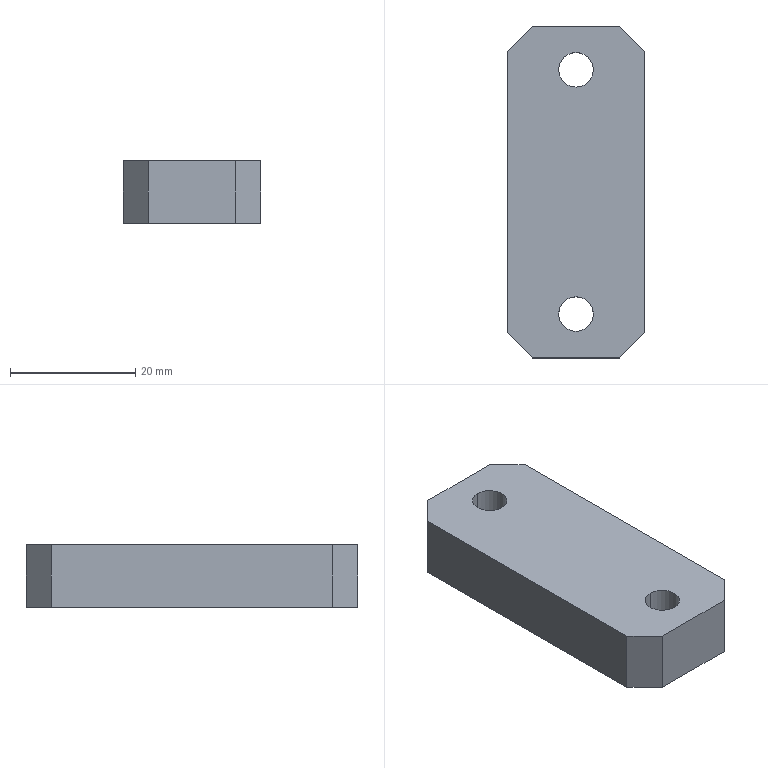Part | Creo | 1 solid | 20 faces | box 22 x 53 x 10 mm | volume 10299 mm3 | plane 12 | cylinder 8 | commonest cylinder face diameters 5.5 x4 9.5 x4
STEP:
#1=CARTESIAN_POINT('',(-173.234,182.442,-294.5));
#2=VERTEX_POINT('',#1);
#3=CARTESIAN_POINT('',(-173.234,227.442,-294.5));
#4=VERTEX_POINT('',#3);
#5=CARTESIAN_POINT('',(-173.234,182.442,-294.5));
#6=DIRECTION('',(0.,1.,0.));
#7=VECTOR('',#6,45.);
#8=LINE('',#5,#7);
#9=EDGE_CURVE('',#2,#4,#8,.T.);
#10=ORIENTED_EDGE('',*,*,#9,.F.);
#11=CARTESIAN_POINT('',(-177.234,178.442,-294.5));
#12=VERTEX_POINT('',#11);
#13=CARTESIAN_POINT('',(-177.234,178.442,-294.5));
#14=DIRECTION('',(0.7071,0.7071,0.));
#15=VECTOR('',#14,5.657);
#16=LINE('',#13,#15);
#17=EDGE_CURVE('',#12,#2,#16,.T.);
#18=ORIENTED_EDGE('',*,*,#17,.F.);
#19=CARTESIAN_POINT('',(-191.234,178.442,-294.5));
#20=VERTEX_POINT('',#19);
#21=CARTESIAN_POINT('',(-177.234,178.442,-294.5));
#22=DIRECTION('',(-1.,0.,0.));
#23=VECTOR('',#22,14.);
#24=LINE('',#21,#23);
#25=EDGE_CURVE('',#12,#20,#24,.T.);
#26=ORIENTED_EDGE('',*,*,#25,.T.);
#27=CARTESIAN_POINT('',(-195.234,182.442,-294.5));
#28=VERTEX_POINT('',#27);
#29=CARTESIAN_POINT('',(-195.234,182.442,-294.5));
#30=DIRECTION('',(0.7071,-0.7071,0.));
#31=VECTOR('',#30,5.657);
#32=LINE('',#29,#31);
#33=EDGE_CURVE('',#28,#20,#32,.T.);
#34=ORIENTED_EDGE('',*,*,#33,.F.);
#35=CARTESIAN_POINT('',(-195.234,227.442,-294.5));
#36=VERTEX_POINT('',#35);
#37=CARTESIAN_POINT('',(-195.234,227.442,-294.5));
#38=DIRECTION('',(0.,-1.,0.));
#39=VECTOR('',#38,45.);
#40=LINE('',#37,#39);
#41=EDGE_CURVE('',#36,#28,#40,.T.);
#42=ORIENTED_EDGE('',*,*,#41,.F.);
#43=CARTESIAN_POINT('',(-191.234,231.442,-294.5));
#44=VERTEX_POINT('',#43);
#45=CARTESIAN_POINT('',(-191.234,231.442,-294.5));
#46=DIRECTION('',(-0.7071,-0.7071,0.));
#47=VECTOR('',#46,5.657);
#48=LINE('',#45,#47);
#49=EDGE_CURVE('',#44,#36,#48,.T.);
#50=ORIENTED_EDGE('',*,*,#49,.F.);
#51=CARTESIAN_POINT('',(-177.234,231.442,-294.5));
#52=VERTEX_POINT('',#51);
#53=CARTESIAN_POINT('',(-177.234,231.442,-294.5));
#54=DIRECTION('',(-1.,0.,0.));
#55=VECTOR('',#54,14.);
#56=LINE('',#53,#55);
#57=EDGE_CURVE('',#52,#44,#56,.T.);
#58=ORIENTED_EDGE('',*,*,#57,.F.);
#59=CARTESIAN_POINT('',(-173.234,227.442,-294.5));
#60=DIRECTION('',(-0.7071,0.7071,0.));
#61=VECTOR('',#60,5.657);
#62=LINE('',#59,#61);
#63=EDGE_CURVE('',#4,#52,#62,.T.);
#64=ORIENTED_EDGE('',*,*,#63,.F.);
#65=EDGE_LOOP('',(#10,#18,#26,#34,#42,#50,#58,#64));
#66=FACE_OUTER_BOUND('',#65,.F.);
#67=CARTESIAN_POINT('',(-184.234,188.192,-294.5));
#68=VERTEX_POINT('',#67);
#69=CARTESIAN_POINT('',(-184.234,182.692,-294.5));
#70=VERTEX_POINT('',#69);
#71=CARTESIAN_POINT('',(-184.234,185.442,-294.5));
#72=DIRECTION('',(0.,0.,-1.));
#73=DIRECTION('',(0.,1.,0.));
#74=AXIS2_PLACEMENT_3D('',#71,#72,#73);
#75=CIRCLE('',#74,2.75);
#76=EDGE_CURVE('',#68,#70,#75,.T.);
#77=ORIENTED_EDGE('',*,*,#76,.F.);
#78=CARTESIAN_POINT('',(-184.234,185.442,-294.5));
#79=DIRECTION('',(0.,0.,-1.));
#80=DIRECTION('',(0.,-1.,0.));
#81=AXIS2_PLACEMENT_3D('',#78,#79,#80);
#82=CIRCLE('',#81,2.75);
#83=EDGE_CURVE('',#70,#68,#82,.T.);
#84=ORIENTED_EDGE('',*,*,#83,.F.);
#85=EDGE_LOOP('',(#77,#84));
#86=FACE_BOUND('',#85,.F.);
#87=CARTESIAN_POINT('',(-184.234,227.192,-294.5));
#88=VERTEX_POINT('',#87);
#89=CARTESIAN_POINT('',(-184.234,221.692,-294.5));
#90=VERTEX_POINT('',#89);
#91=CARTESIAN_POINT('',(-184.234,224.442,-294.5));
#92=DIRECTION('',(0.,0.,-1.));
#93=DIRECTION('',(0.,1.,0.));
#94=AXIS2_PLACEMENT_3D('',#91,#92,#93);
#95=CIRCLE('',#94,2.75);
#96=EDGE_CURVE('',#88,#90,#95,.T.);
#97=ORIENTED_EDGE('',*,*,#96,.F.);
#98=CARTESIAN_POINT('',(-184.234,224.442,-294.5));
#99=DIRECTION('',(0.,0.,-1.));
#100=DIRECTION('',(0.,-1.,0.));
#101=AXIS2_PLACEMENT_3D('',#98,#99,#100);
#102=CIRCLE('',#101,2.75);
#103=EDGE_CURVE('',#90,#88,#102,.T.);
#104=ORIENTED_EDGE('',*,*,#103,.F.);
#105=EDGE_LOOP('',(#97,#104));
#106=FACE_BOUND('',#105,.F.);
#107=CARTESIAN_POINT('',(-194.234,202.392,-294.5));
#108=DIRECTION('',(0.,0.,1.));
#109=DIRECTION('',(0.,-1.,0.));
#110=AXIS2_PLACEMENT_3D('',#107,#108,#109);
#111=PLANE('',#110);
#112=ADVANCED_FACE('',(#66,#86,#106),#111,.T.);
#113=CARTESIAN_POINT('',(-173.234,227.442,-304.5));
#114=VERTEX_POINT('',#113);
#115=CARTESIAN_POINT('',(-173.234,182.442,-304.5));
#116=VERTEX_POINT('',#115);
#117=CARTESIAN_POINT('',(-173.234,227.442,-304.5));
#118=DIRECTION('',(0.,-1.,0.));
#119=VECTOR('',#118,45.);
#120=LINE('',#117,#119);
#121=EDGE_CURVE('',#114,#116,#120,.T.);
#122=ORIENTED_EDGE('',*,*,#121,.T.);
#123=CARTESIAN_POINT('',(-173.234,182.442,-294.5));
#124=DIRECTION('',(0.,0.,-1.));
#125=VECTOR('',#124,10.);
#126=LINE('',#123,#125);
#127=EDGE_CURVE('',#2,#116,#126,.T.);
#128=ORIENTED_EDGE('',*,*,#127,.F.);
#129=ORIENTED_EDGE('',*,*,#9,.T.);
#130=CARTESIAN_POINT('',(-173.234,227.442,-304.5));
#131=DIRECTION('',(0.,0.,1.));
#132=VECTOR('',#131,10.);
#133=LINE('',#130,#132);
#134=EDGE_CURVE('',#114,#4,#133,.T.);
#135=ORIENTED_EDGE('',*,*,#134,.F.);
#136=EDGE_LOOP('',(#122,#128,#129,#135));
#137=FACE_OUTER_BOUND('',#136,.F.);
#138=CARTESIAN_POINT('',(-173.234,184.642,-299.5));
#139=DIRECTION('',(-1.,0.,0.));
#140=DIRECTION('',(0.,0.,1.));
#141=AXIS2_PLACEMENT_3D('',#138,#139,#140);
#142=PLANE('',#141);
#143=ADVANCED_FACE('',(#137),#142,.F.);
#144=CARTESIAN_POINT('',(-195.234,182.442,-304.5));
#145=VERTEX_POINT('',#144);
#146=CARTESIAN_POINT('',(-195.234,227.442,-304.5));
#147=VERTEX_POINT('',#146);
#148=CARTESIAN_POINT('',(-195.234,182.442,-304.5));
#149=DIRECTION('',(0.,1.,0.));
#150=VECTOR('',#149,45.);
#151=LINE('',#148,#150);
#152=EDGE_CURVE('',#145,#147,#151,.T.);
#153=ORIENTED_EDGE('',*,*,#152,.F.);
#154=CARTESIAN_POINT('',(-191.234,178.442,-304.5));
#155=VERTEX_POINT('',#154);
#156=CARTESIAN_POINT('',(-191.234,178.442,-304.5));
#157=DIRECTION('',(-0.7071,0.7071,0.));
#158=VECTOR('',#157,5.657);
#159=LINE('',#156,#158);
#160=EDGE_CURVE('',#155,#145,#159,.T.);
#161=ORIENTED_EDGE('',*,*,#160,.F.);
#162=CARTESIAN_POINT('',(-177.234,178.442,-304.5));
#163=VERTEX_POINT('',#162);
#164=CARTESIAN_POINT('',(-191.234,178.442,-304.5));
#165=DIRECTION('',(1.,0.,0.));
#166=VECTOR('',#165,14.);
#167=LINE('',#164,#166);
#168=EDGE_CURVE('',#155,#163,#167,.T.);
#169=ORIENTED_EDGE('',*,*,#168,.T.);
#170=CARTESIAN_POINT('',(-173.234,182.442,-304.5));
#171=DIRECTION('',(-0.7071,-0.7071,0.));
#172=VECTOR('',#171,5.657);
#173=LINE('',#170,#172);
#174=EDGE_CURVE('',#116,#163,#173,.T.);
#175=ORIENTED_EDGE('',*,*,#174,.F.);
#176=ORIENTED_EDGE('',*,*,#121,.F.);
#177=CARTESIAN_POINT('',(-177.234,231.442,-304.5));
#178=VERTEX_POINT('',#177);
#179=CARTESIAN_POINT('',(-177.234,231.442,-304.5));
#180=DIRECTION('',(0.7071,-0.7071,0.));
#181=VECTOR('',#180,5.657);
#182=LINE('',#179,#181);
#183=EDGE_CURVE('',#178,#114,#182,.T.);
#184=ORIENTED_EDGE('',*,*,#183,.F.);
#185=CARTESIAN_POINT('',(-191.234,231.442,-304.5));
#186=VERTEX_POINT('',#185);
#187=CARTESIAN_POINT('',(-191.234,231.442,-304.5));
#188=DIRECTION('',(1.,0.,0.));
#189=VECTOR('',#188,14.);
#190=LINE('',#187,#189);
#191=EDGE_CURVE('',#186,#178,#190,.T.);
#192=ORIENTED_EDGE('',*,*,#191,.F.);
#193=CARTESIAN_POINT('',(-195.234,227.442,-304.5));
#194=DIRECTION('',(0.7071,0.7071,0.));
#195=VECTOR('',#194,5.657);
#196=LINE('',#193,#195);
#197=EDGE_CURVE('',#147,#186,#196,.T.);
#198=ORIENTED_EDGE('',*,*,#197,.F.);
#199=EDGE_LOOP('',(#153,#161,#169,#175,#176,#184,#192,#198));
#200=FACE_OUTER_BOUND('',#199,.F.);
#201=CARTESIAN_POINT('',(-184.234,190.192,-304.5));
#202=VERTEX_POINT('',#201);
#203=CARTESIAN_POINT('',(-184.234,180.692,-304.5));
#204=VERTEX_POINT('',#203);
#205=CARTESIAN_POINT('',(-184.234,185.442,-304.5));
#206=DIRECTION('',(0.,0.,1.));
#207=DIRECTION('',(0.,1.,0.));
#208=AXIS2_PLACEMENT_3D('',#205,#206,#207);
#209=CIRCLE('',#208,4.75);
#210=EDGE_CURVE('',#202,#204,#209,.T.);
#211=ORIENTED_EDGE('',*,*,#210,.F.);
#212=CARTESIAN_POINT('',(-184.234,185.442,-304.5));
#213=DIRECTION('',(0.,0.,1.));
#214=DIRECTION('',(0.,-1.,0.));
#215=AXIS2_PLACEMENT_3D('',#212,#213,#214);
#216=CIRCLE('',#215,4.75);
#217=EDGE_CURVE('',#204,#202,#216,.T.);
#218=ORIENTED_EDGE('',*,*,#217,.F.);
#219=EDGE_LOOP('',(#211,#218));
#220=FACE_BOUND('',#219,.F.);
#221=CARTESIAN_POINT('',(-184.234,229.192,-304.5));
#222=VERTEX_POINT('',#221);
#223=CARTESIAN_POINT('',(-184.234,219.692,-304.5));
#224=VERTEX_POINT('',#223);
#225=CARTESIAN_POINT('',(-184.234,224.442,-304.5));
#226=DIRECTION('',(0.,0.,1.));
#227=DIRECTION('',(0.,1.,0.));
#228=AXIS2_PLACEMENT_3D('',#225,#226,#227);
#229=CIRCLE('',#228,4.75);
#230=EDGE_CURVE('',#222,#224,#229,.T.);
#231=ORIENTED_EDGE('',*,*,#230,.F.);
#232=CARTESIAN_POINT('',(-184.234,224.442,-304.5));
#233=DIRECTION('',(0.,0.,1.));
#234=DIRECTION('',(0.,-1.,0.));
#235=AXIS2_PLACEMENT_3D('',#232,#233,#234);
#236=CIRCLE('',#235,4.75);
#237=EDGE_CURVE('',#224,#222,#236,.T.);
#238=ORIENTED_EDGE('',*,*,#237,.F.);
#239=EDGE_LOOP('',(#231,#238));
#240=FACE_BOUND('',#239,.F.);
#241=CARTESIAN_POINT('',(-194.234,202.392,-304.5));
#242=DIRECTION('',(0.,0.,-1.));
#243=DIRECTION('',(0.,1.,0.));
#244=AXIS2_PLACEMENT_3D('',#241,#242,#243);
#245=PLANE('',#244);
#246=ADVANCED_FACE('',(#200,#220,#240),#245,.T.);
#247=ORIENTED_EDGE('',*,*,#41,.T.);
#248=CARTESIAN_POINT('',(-195.234,182.442,-304.5));
#249=DIRECTION('',(0.,0.,1.));
#250=VECTOR('',#249,10.);
#251=LINE('',#248,#250);
#252=EDGE_CURVE('',#145,#28,#251,.T.);
#253=ORIENTED_EDGE('',*,*,#252,.F.);
#254=ORIENTED_EDGE('',*,*,#152,.T.);
#255=CARTESIAN_POINT('',(-195.234,227.442,-294.5));
#256=DIRECTION('',(0.,0.,-1.));
#257=VECTOR('',#256,10.);
#258=LINE('',#255,#257);
#259=EDGE_CURVE('',#36,#147,#258,.T.);
#260=ORIENTED_EDGE('',*,*,#259,.F.);
#261=EDGE_LOOP('',(#247,#253,#254,#260));
#262=FACE_OUTER_BOUND('',#261,.F.);
#263=CARTESIAN_POINT('',(-195.234,207.142,-299.5));
#264=DIRECTION('',(1.,0.,0.));
#265=DIRECTION('',(0.,0.,1.));
#266=AXIS2_PLACEMENT_3D('',#263,#264,#265);
#267=PLANE('',#266);
#268=ADVANCED_FACE('',(#262),#267,.F.);
#269=ORIENTED_EDGE('',*,*,#160,.T.);
#270=ORIENTED_EDGE('',*,*,#252,.T.);
#271=ORIENTED_EDGE('',*,*,#33,.T.);
#272=CARTESIAN_POINT('',(-191.234,178.442,-294.5));
#273=DIRECTION('',(0.,0.,-1.));
#274=VECTOR('',#273,10.);
#275=LINE('',#272,#274);
#276=EDGE_CURVE('',#20,#155,#275,.T.);
#277=ORIENTED_EDGE('',*,*,#276,.T.);
#278=EDGE_LOOP('',(#269,#270,#271,#277));
#279=FACE_OUTER_BOUND('',#278,.F.);
#280=CARTESIAN_POINT('',(-191.234,178.442,-299.5));
#281=DIRECTION('',(0.7071,0.7071,0.));
#282=DIRECTION('',(0.7071,-0.7071,0.));
#283=AXIS2_PLACEMENT_3D('',#280,#281,#282);
#284=PLANE('',#283);
#285=ADVANCED_FACE('',(#279),#284,.F.);
#286=ORIENTED_EDGE('',*,*,#25,.F.);
#287=CARTESIAN_POINT('',(-177.234,178.442,-304.5));
#288=DIRECTION('',(0.,0.,1.));
#289=VECTOR('',#288,10.);
#290=LINE('',#287,#289);
#291=EDGE_CURVE('',#163,#12,#290,.T.);
#292=ORIENTED_EDGE('',*,*,#291,.F.);
#293=ORIENTED_EDGE('',*,*,#168,.F.);
#294=ORIENTED_EDGE('',*,*,#276,.F.);
#295=EDGE_LOOP('',(#286,#292,#293,#294));
#296=FACE_OUTER_BOUND('',#295,.F.);
#297=CARTESIAN_POINT('',(-196.234,178.442,-299.5));
#298=DIRECTION('',(0.,1.,0.));
#299=DIRECTION('',(0.,0.,-1.));
#300=AXIS2_PLACEMENT_3D('',#297,#298,#299);
#301=PLANE('',#300);
#302=ADVANCED_FACE('',(#296),#301,.F.);
#303=ORIENTED_EDGE('',*,*,#174,.T.);
#304=ORIENTED_EDGE('',*,*,#291,.T.);
#305=ORIENTED_EDGE('',*,*,#17,.T.);
#306=ORIENTED_EDGE('',*,*,#127,.T.);
#307=EDGE_LOOP('',(#303,#304,#305,#306));
#308=FACE_OUTER_BOUND('',#307,.F.);
#309=CARTESIAN_POINT('',(-173.234,182.442,-299.5));
#310=DIRECTION('',(-0.7071,0.7071,0.));
#311=DIRECTION('',(0.7071,0.7071,0.));
#312=AXIS2_PLACEMENT_3D('',#309,#310,#311);
#313=PLANE('',#312);
#314=ADVANCED_FACE('',(#308),#313,.F.);
#315=ORIENTED_EDGE('',*,*,#197,.T.);
#316=CARTESIAN_POINT('',(-191.234,231.442,-304.5));
#317=DIRECTION('',(0.,0.,1.));
#318=VECTOR('',#317,10.);
#319=LINE('',#316,#318);
#320=EDGE_CURVE('',#186,#44,#319,.T.);
#321=ORIENTED_EDGE('',*,*,#320,.T.);
#322=ORIENTED_EDGE('',*,*,#49,.T.);
#323=ORIENTED_EDGE('',*,*,#259,.T.);
#324=EDGE_LOOP('',(#315,#321,#322,#323));
#325=FACE_OUTER_BOUND('',#324,.F.);
#326=CARTESIAN_POINT('',(-195.234,227.442,-299.5));
#327=DIRECTION('',(0.7071,-0.7071,0.));
#328=DIRECTION('',(-0.7071,-0.7071,0.));
#329=AXIS2_PLACEMENT_3D('',#326,#327,#328);
#330=PLANE('',#329);
#331=ADVANCED_FACE('',(#325),#330,.F.);
#332=ORIENTED_EDGE('',*,*,#57,.T.);
#333=ORIENTED_EDGE('',*,*,#320,.F.);
#334=ORIENTED_EDGE('',*,*,#191,.T.);
#335=CARTESIAN_POINT('',(-177.234,231.442,-294.5));
#336=DIRECTION('',(0.,0.,-1.));
#337=VECTOR('',#336,10.);
#338=LINE('',#335,#337);
#339=EDGE_CURVE('',#52,#178,#338,.T.);
#340=ORIENTED_EDGE('',*,*,#339,.F.);
#341=EDGE_LOOP('',(#332,#333,#334,#340));
#342=FACE_OUTER_BOUND('',#341,.F.);
#343=CARTESIAN_POINT('',(-196.234,231.442,-299.5));
#344=DIRECTION('',(0.,-1.,0.));
#345=DIRECTION('',(0.,0.,-1.));
#346=AXIS2_PLACEMENT_3D('',#343,#344,#345);
#347=PLANE('',#346);
#348=ADVANCED_FACE('',(#342),#347,.F.);
#349=ORIENTED_EDGE('',*,*,#183,.T.);
#350=ORIENTED_EDGE('',*,*,#134,.T.);
#351=ORIENTED_EDGE('',*,*,#63,.T.);
#352=ORIENTED_EDGE('',*,*,#339,.T.);
#353=EDGE_LOOP('',(#349,#350,#351,#352));
#354=FACE_OUTER_BOUND('',#353,.F.);
#355=CARTESIAN_POINT('',(-177.234,231.442,-299.5));
#356=DIRECTION('',(-0.7071,-0.7071,0.));
#357=DIRECTION('',(-0.7071,0.7071,0.));
#358=AXIS2_PLACEMENT_3D('',#355,#356,#357);
#359=PLANE('',#358);
#360=ADVANCED_FACE('',(#354),#359,.F.);
#361=ORIENTED_EDGE('',*,*,#210,.T.);
#362=CARTESIAN_POINT('',(-184.234,180.692,-298.5));
#363=VERTEX_POINT('',#362);
#364=CARTESIAN_POINT('',(-184.234,180.692,-298.5));
#365=DIRECTION('',(0.,0.,-1.));
#366=VECTOR('',#365,6.);
#367=LINE('',#364,#366);
#368=EDGE_CURVE('',#363,#204,#367,.T.);
#369=ORIENTED_EDGE('',*,*,#368,.F.);
#370=CARTESIAN_POINT('',(-184.234,190.192,-298.5));
#371=VERTEX_POINT('',#370);
#372=CARTESIAN_POINT('',(-184.234,185.442,-298.5));
#373=DIRECTION('',(0.,0.,-1.));
#374=DIRECTION('',(0.,-1.,0.));
#375=AXIS2_PLACEMENT_3D('',#372,#373,#374);
#376=CIRCLE('',#375,4.75);
#377=EDGE_CURVE('',#363,#371,#376,.T.);
#378=ORIENTED_EDGE('',*,*,#377,.T.);
#379=CARTESIAN_POINT('',(-184.234,190.192,-298.5));
#380=DIRECTION('',(0.,0.,-1.));
#381=VECTOR('',#380,6.);
#382=LINE('',#379,#381);
#383=EDGE_CURVE('',#371,#202,#382,.T.);
#384=ORIENTED_EDGE('',*,*,#383,.T.);
#385=EDGE_LOOP('',(#361,#369,#378,#384));
#386=FACE_OUTER_BOUND('',#385,.F.);
#387=CARTESIAN_POINT('',(-184.234,185.442,-298.5));
#388=DIRECTION('',(0.,0.,-1.));
#389=DIRECTION('',(0.,1.,0.));
#390=AXIS2_PLACEMENT_3D('',#387,#388,#389);
#391=CYLINDRICAL_SURFACE('',#390,4.75);
#392=ADVANCED_FACE('',(#386),#391,.F.);
#393=ORIENTED_EDGE('',*,*,#217,.T.);
#394=ORIENTED_EDGE('',*,*,#383,.F.);
#395=CARTESIAN_POINT('',(-184.234,185.442,-298.5));
#396=DIRECTION('',(0.,0.,-1.));
#397=DIRECTION('',(0.,1.,0.));
#398=AXIS2_PLACEMENT_3D('',#395,#396,#397);
#399=CIRCLE('',#398,4.75);
#400=EDGE_CURVE('',#371,#363,#399,.T.);
#401=ORIENTED_EDGE('',*,*,#400,.T.);
#402=ORIENTED_EDGE('',*,*,#368,.T.);
#403=EDGE_LOOP('',(#393,#394,#401,#402));
#404=FACE_OUTER_BOUND('',#403,.F.);
#405=CARTESIAN_POINT('',(-184.234,185.442,-298.5));
#406=DIRECTION('',(0.,0.,-1.));
#407=DIRECTION('',(0.,1.,0.));
#408=AXIS2_PLACEMENT_3D('',#405,#406,#407);
#409=CYLINDRICAL_SURFACE('',#408,4.75);
#410=ADVANCED_FACE('',(#404),#409,.F.);
#411=ORIENTED_EDGE('',*,*,#400,.F.);
#412=ORIENTED_EDGE('',*,*,#377,.F.);
#413=EDGE_LOOP('',(#411,#412));
#414=FACE_OUTER_BOUND('',#413,.F.);
#415=CARTESIAN_POINT('',(-184.234,188.192,-298.5));
#416=VERTEX_POINT('',#415);
#417=CARTESIAN_POINT('',(-184.234,182.692,-298.5));
#418=VERTEX_POINT('',#417);
#419=CARTESIAN_POINT('',(-184.234,185.442,-298.5));
#420=DIRECTION('',(0.,0.,1.));
#421=DIRECTION('',(0.,1.,0.));
#422=AXIS2_PLACEMENT_3D('',#419,#420,#421);
#423=CIRCLE('',#422,2.75);
#424=EDGE_CURVE('',#416,#418,#423,.T.);
#425=ORIENTED_EDGE('',*,*,#424,.F.);
#426=CARTESIAN_POINT('',(-184.234,185.442,-298.5));
#427=DIRECTION('',(0.,0.,1.));
#428=DIRECTION('',(0.,-1.,0.));
#429=AXIS2_PLACEMENT_3D('',#426,#427,#428);
#430=CIRCLE('',#429,2.75);
#431=EDGE_CURVE('',#418,#416,#430,.T.);
#432=ORIENTED_EDGE('',*,*,#431,.F.);
#433=EDGE_LOOP('',(#425,#432));
#434=FACE_BOUND('',#433,.F.);
#435=CARTESIAN_POINT('',(-184.234,185.442,-298.5));
#436=DIRECTION('',(0.,0.,1.));
#437=DIRECTION('',(0.,-1.,0.));
#438=AXIS2_PLACEMENT_3D('',#435,#436,#437);
#439=PLANE('',#438);
#440=ADVANCED_FACE('',(#414,#434),#439,.F.);
#441=ORIENTED_EDGE('',*,*,#424,.T.);
#442=CARTESIAN_POINT('',(-184.234,182.692,-294.5));
#443=DIRECTION('',(0.,0.,-1.));
#444=VECTOR('',#443,4.);
#445=LINE('',#442,#444);
#446=EDGE_CURVE('',#70,#418,#445,.T.);
#447=ORIENTED_EDGE('',*,*,#446,.F.);
#448=ORIENTED_EDGE('',*,*,#83,.T.);
#449=CARTESIAN_POINT('',(-184.234,188.192,-294.5));
#450=DIRECTION('',(0.,0.,-1.));
#451=VECTOR('',#450,4.);
#452=LINE('',#449,#451);
#453=EDGE_CURVE('',#68,#416,#452,.T.);
#454=ORIENTED_EDGE('',*,*,#453,.T.);
#455=EDGE_LOOP('',(#441,#447,#448,#454));
#456=FACE_OUTER_BOUND('',#455,.F.);
#457=CARTESIAN_POINT('',(-184.234,185.442,-294.5));
#458=DIRECTION('',(0.,0.,-1.));
#459=DIRECTION('',(0.,1.,0.));
#460=AXIS2_PLACEMENT_3D('',#457,#458,#459);
#461=CYLINDRICAL_SURFACE('',#460,2.75);
#462=ADVANCED_FACE('',(#456),#461,.F.);
#463=ORIENTED_EDGE('',*,*,#431,.T.);
#464=ORIENTED_EDGE('',*,*,#453,.F.);
#465=ORIENTED_EDGE('',*,*,#76,.T.);
#466=ORIENTED_EDGE('',*,*,#446,.T.);
#467=EDGE_LOOP('',(#463,#464,#465,#466));
#468=FACE_OUTER_BOUND('',#467,.F.);
#469=CARTESIAN_POINT('',(-184.234,185.442,-294.5));
#470=DIRECTION('',(0.,0.,-1.));
#471=DIRECTION('',(0.,1.,0.));
#472=AXIS2_PLACEMENT_3D('',#469,#470,#471);
#473=CYLINDRICAL_SURFACE('',#472,2.75);
#474=ADVANCED_FACE('',(#468),#473,.F.);
#475=ORIENTED_EDGE('',*,*,#230,.T.);
#476=CARTESIAN_POINT('',(-184.234,219.692,-298.5));
#477=VERTEX_POINT('',#476);
#478=CARTESIAN_POINT('',(-184.234,219.692,-298.5));
#479=DIRECTION('',(0.,0.,-1.));
#480=VECTOR('',#479,6.);
#481=LINE('',#478,#480);
#482=EDGE_CURVE('',#477,#224,#481,.T.);
#483=ORIENTED_EDGE('',*,*,#482,.F.);
#484=CARTESIAN_POINT('',(-184.234,229.192,-298.5));
#485=VERTEX_POINT('',#484);
#486=CARTESIAN_POINT('',(-184.234,224.442,-298.5));
#487=DIRECTION('',(0.,0.,-1.));
#488=DIRECTION('',(0.,-1.,0.));
#489=AXIS2_PLACEMENT_3D('',#486,#487,#488);
#490=CIRCLE('',#489,4.75);
#491=EDGE_CURVE('',#477,#485,#490,.T.);
#492=ORIENTED_EDGE('',*,*,#491,.T.);
#493=CARTESIAN_POINT('',(-184.234,229.192,-298.5));
#494=DIRECTION('',(0.,0.,-1.));
#495=VECTOR('',#494,6.);
#496=LINE('',#493,#495);
#497=EDGE_CURVE('',#485,#222,#496,.T.);
#498=ORIENTED_EDGE('',*,*,#497,.T.);
#499=EDGE_LOOP('',(#475,#483,#492,#498));
#500=FACE_OUTER_BOUND('',#499,.F.);
#501=CARTESIAN_POINT('',(-184.234,224.442,-298.5));
#502=DIRECTION('',(0.,0.,-1.));
#503=DIRECTION('',(0.,1.,0.));
#504=AXIS2_PLACEMENT_3D('',#501,#502,#503);
#505=CYLINDRICAL_SURFACE('',#504,4.75);
#506=ADVANCED_FACE('',(#500),#505,.F.);
#507=ORIENTED_EDGE('',*,*,#237,.T.);
#508=ORIENTED_EDGE('',*,*,#497,.F.);
#509=CARTESIAN_POINT('',(-184.234,224.442,-298.5));
#510=DIRECTION('',(0.,0.,-1.));
#511=DIRECTION('',(0.,1.,0.));
#512=AXIS2_PLACEMENT_3D('',#509,#510,#511);
#513=CIRCLE('',#512,4.75);
#514=EDGE_CURVE('',#485,#477,#513,.T.);
#515=ORIENTED_EDGE('',*,*,#514,.T.);
#516=ORIENTED_EDGE('',*,*,#482,.T.);
#517=EDGE_LOOP('',(#507,#508,#515,#516));
#518=FACE_OUTER_BOUND('',#517,.F.);
#519=CARTESIAN_POINT('',(-184.234,224.442,-298.5));
#520=DIRECTION('',(0.,0.,-1.));
#521=DIRECTION('',(0.,1.,0.));
#522=AXIS2_PLACEMENT_3D('',#519,#520,#521);
#523=CYLINDRICAL_SURFACE('',#522,4.75);
#524=ADVANCED_FACE('',(#518),#523,.F.);
#525=ORIENTED_EDGE('',*,*,#514,.F.);
#526=ORIENTED_EDGE('',*,*,#491,.F.);
#527=EDGE_LOOP('',(#525,#526));
#528=FACE_OUTER_BOUND('',#527,.F.);
#529=CARTESIAN_POINT('',(-184.234,227.192,-298.5));
#530=VERTEX_POINT('',#529);
#531=CARTESIAN_POINT('',(-184.234,221.692,-298.5));
#532=VERTEX_POINT('',#531);
#533=CARTESIAN_POINT('',(-184.234,224.442,-298.5));
#534=DIRECTION('',(0.,0.,1.));
#535=DIRECTION('',(0.,1.,0.));
#536=AXIS2_PLACEMENT_3D('',#533,#534,#535);
#537=CIRCLE('',#536,2.75);
#538=EDGE_CURVE('',#530,#532,#537,.T.);
#539=ORIENTED_EDGE('',*,*,#538,.F.);
#540=CARTESIAN_POINT('',(-184.234,224.442,-298.5));
#541=DIRECTION('',(0.,0.,1.));
#542=DIRECTION('',(0.,-1.,0.));
#543=AXIS2_PLACEMENT_3D('',#540,#541,#542);
#544=CIRCLE('',#543,2.75);
#545=EDGE_CURVE('',#532,#530,#544,.T.);
#546=ORIENTED_EDGE('',*,*,#545,.F.);
#547=EDGE_LOOP('',(#539,#546));
#548=FACE_BOUND('',#547,.F.);
#549=CARTESIAN_POINT('',(-184.234,224.442,-298.5));
#550=DIRECTION('',(0.,0.,1.));
#551=DIRECTION('',(0.,-1.,0.));
#552=AXIS2_PLACEMENT_3D('',#549,#550,#551);
#553=PLANE('',#552);
#554=ADVANCED_FACE('',(#528,#548),#553,.F.);
#555=ORIENTED_EDGE('',*,*,#538,.T.);
#556=CARTESIAN_POINT('',(-184.234,221.692,-294.5));
#557=DIRECTION('',(0.,0.,-1.));
#558=VECTOR('',#557,4.);
#559=LINE('',#556,#558);
#560=EDGE_CURVE('',#90,#532,#559,.T.);
#561=ORIENTED_EDGE('',*,*,#560,.F.);
#562=ORIENTED_EDGE('',*,*,#103,.T.);
#563=CARTESIAN_POINT('',(-184.234,227.192,-294.5));
#564=DIRECTION('',(0.,0.,-1.));
#565=VECTOR('',#564,4.);
#566=LINE('',#563,#565);
#567=EDGE_CURVE('',#88,#530,#566,.T.);
#568=ORIENTED_EDGE('',*,*,#567,.T.);
#569=EDGE_LOOP('',(#555,#561,#562,#568));
#570=FACE_OUTER_BOUND('',#569,.F.);
#571=CARTESIAN_POINT('',(-184.234,224.442,-294.5));
#572=DIRECTION('',(0.,0.,-1.));
#573=DIRECTION('',(0.,1.,0.));
#574=AXIS2_PLACEMENT_3D('',#571,#572,#573);
#575=CYLINDRICAL_SURFACE('',#574,2.75);
#576=ADVANCED_FACE('',(#570),#575,.F.);
#577=ORIENTED_EDGE('',*,*,#545,.T.);
#578=ORIENTED_EDGE('',*,*,#567,.F.);
#579=ORIENTED_EDGE('',*,*,#96,.T.);
#580=ORIENTED_EDGE('',*,*,#560,.T.);
#581=EDGE_LOOP('',(#577,#578,#579,#580));
#582=FACE_OUTER_BOUND('',#581,.F.);
#583=CARTESIAN_POINT('',(-184.234,224.442,-294.5));
#584=DIRECTION('',(0.,0.,-1.));
#585=DIRECTION('',(0.,1.,0.));
#586=AXIS2_PLACEMENT_3D('',#583,#584,#585);
#587=CYLINDRICAL_SURFACE('',#586,2.75);
#588=ADVANCED_FACE('',(#582),#587,.F.);
#589=CLOSED_SHELL('',(#112,#143,#246,#268,#285,#302,#314,#331,#348,#360,#392,#410,#440,#462,#474,#506,#524,#554,#576,#588));
#590=MANIFOLD_SOLID_BREP('',#589);
#591=(LENGTH_UNIT()NAMED_UNIT(*)SI_UNIT(.MILLI.,.METRE.));
#592=UNCERTAINTY_MEASURE_WITH_UNIT(LENGTH_MEASURE(0.005825),#591,'','');
#593=(NAMED_UNIT(*)PLANE_ANGLE_UNIT()SI_UNIT($,.RADIAN.));
#594=PLANE_ANGLE_MEASURE_WITH_UNIT(PLANE_ANGLE_MEASURE(0.01745),#593);
#595=(CONVERSION_BASED_UNIT('DEGREE',#594)NAMED_UNIT(*)PLANE_ANGLE_UNIT());
#596=(NAMED_UNIT(*)SI_UNIT($,.STERADIAN.)SOLID_ANGLE_UNIT());
#597=(GEOMETRIC_REPRESENTATION_CONTEXT(3)GLOBAL_UNCERTAINTY_ASSIGNED_CONTEXT((#592))GLOBAL_UNIT_ASSIGNED_CONTEXT((#591,#595,#596))REPRESENTATION_CONTEXT('',''));
#598=ADVANCED_BREP_SHAPE_REPRESENTATION('',(#590),#597);